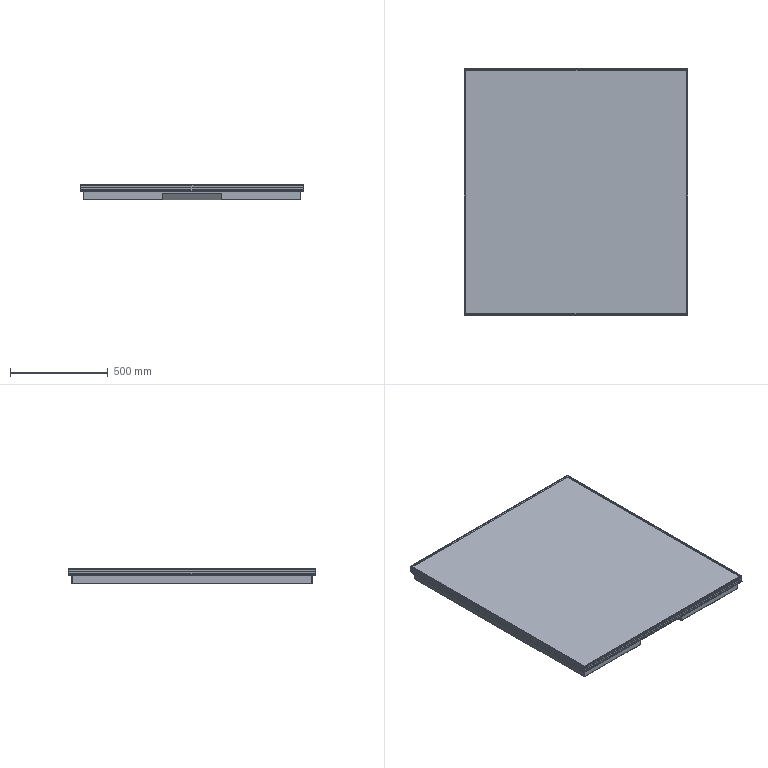Part | SolidWorks | 8 solids | 408 faces | box 1140 x 1260 x 80 mm | volume 7783744 mm3 | plane 254 | cylinder 142 | spline 12 | commonest cylinder face diameters 7 x100 11 x16 1 x9 3 x9 5 x4 0.4 x2